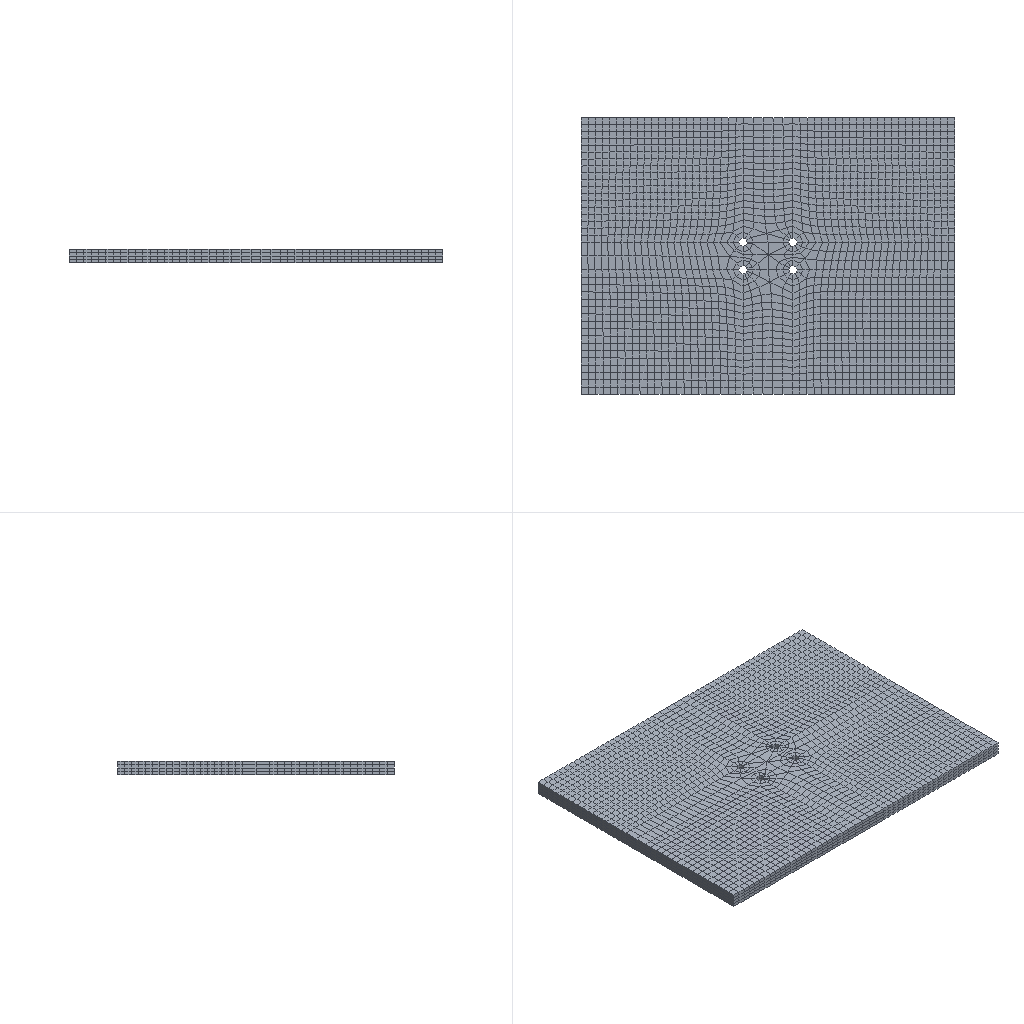Simulation study | abaqus
Set-up summary:
category,name,step,type,value,unit,region
solver,abaqus,,Abaqus/CAE 2024
units,mm-N-s-tonne (MPa),,inferred,E=200000 density=
analysis,Step-1,,static,time_period=1
analysis,Step-2,,static,time_period=1
mesh,nodes,,,10331
mesh,elements,,,7836
element_type,SC8R,,,7836
material,Material-1,,E,200000
material,Material-1,,nu,0.25
material,Material-1,,behaviors,damage initiation; elastic engineering constants
section,,,shell section,1,,CompositeLayup-1-1
load,Load-1,Step-1,pressure,1.977,,_PickedSurf10
load,Load-1-Copy,Step-1,pressure,1.995,,_PickedSurf12
load,Load-1-Copy-Copy,Step-1,pressure,1.934,,_PickedSurf13
load,Load-1-Copy-Copy-Copy,Step-1,pressure,1.945,,_PickedSurf14
load,Load-5,Step-1,pressure,1.974,,_PickedSurf15
load,Load-5-Copy,Step-1,pressure,1.945,,_PickedSurf16
load,Load-5-Copy-Copy,Step-1,pressure,1.995,,_PickedSurf17
load,Load-5-Copy-Copy-Copy,Step-1,pressure,1.934,,_PickedSurf18
bc,BC-1,Step-1,encastre,[dofs=ENCASTRE],,_PickedSet4
bc,BC-2,Step-1,fixed,"[dofs=rx,ry,rz,x,y,z n=6]",,_PickedSet9
bc,BC-2,Step-2,displacement,0.2 [dofs=x],,_PickedSet9
bc,BC-2,Step-2,fixed,"[dofs=rx,ry,rz n=3]",,_PickedSet9
constraint,coupling,,,1
Abaqus input file, long lists of numbers shortened:
*Heading
** Job name: deck Model name: Model-1-Copy-Copy
** Generated by: Abaqus/CAE 2024
*Preprint, echo=NO, model=NO, history=NO, contact=NO
**
** PARTS
**
*Part, name=Part-1
*Node
      1,         156.,         -90.,           0.
      2,         156.,         -90.,          10.
** (10328 more lines like these left out)
*Element, type=SC8R
1,   1,   4, 117, 118, 105, 110, 984, 981
2, 105, 110, 984, 981, 106, 109, 985, 982
** (7834 more lines like these left out)
*Orientation, name=Ori-1
1., 0., 0., 0., 1., 0.
3, 0.
** Region: (CompositeLayup-1-1: Generated From Layup)
*Elset, elset=CompositeLayup-1-1, generate
    1,  7836,     1
** Section: CompositeLayup-1-1
*Shell Section, elset=CompositeLayup-1-1, composite, orientation=Ori-1, stack direction=3, layup=CompositeLayup-1
1., 3, Material-1, -45., Ply-1
1., 3, Material-1, 45., Ply-2
1., 3, Material-1, -45., Ply-3
1., 3, Material-1, 45., Ply-4
*End Part
**
**
** ASSEMBLY
**
*Assembly, name=Assembly
**
*Instance, name=Part-1-1, part=Part-1
*End Instance
**
*Node
      1,         270.,        -100.,           5.
*Nset, nset=_PickedSet4, internal, instance=Part-1-1
   49,   50,   51,   52,   57,   58,   61,   63,  457,  458,  459,  460,  461,  462,  463,  464
  465,  466,  467,  468,  469,  470,  471,  472,  473,  474,  475,  476,  477,  478,  479,  480
** (10 more lines like these left out)
*Elset, elset=_PickedSet4, internal, instance=Part-1-1
 2121, 2122, 2186, 2208, 2213, 2214, 2215, 2216, 2217, 2218, 2219, 2220, 2221, 2222, 2223, 2224
 2225, 2226, 2227, 2228, 2229, 2587, 2588, 2589, 2590, 2591, 2592, 2593, 2594, 2595, 2596, 2597
** (8 more lines like these left out)
*Nset, nset=_PickedSet8, internal
 1,
*Nset, nset=_PickedSet9, internal
 1,
*Elset, elset=__PickedSurf7_S6, internal, instance=Part-1-1
   25,   26,   90,  112, 7541, 7562, 7563, 7564, 7637, 7658, 7679, 7700
*Elset, elset=__PickedSurf7_S3, internal, instance=Part-1-1
 117, 118, 119, 120, 121, 122, 123, 124, 125, 126, 127, 128, 129, 130, 131, 132
 133, 491, 492, 493, 494, 495, 496, 497, 498, 499, 500, 501, 502, 503, 504, 505
** (1 more lines like these left out)
*Elset, elset=__PickedSurf7_S5, internal, instance=Part-1-1
  899,  900,  901,  902,  903,  904,  905,  906,  907,  908,  909,  910,  911,  912,  913,  914
  915,  916,  917,  918,  919,  920,  921,  922,  923,  924,  925,  926,  927,  928,  929,  930
** (5 more lines like these left out)
*Elset, elset=__PickedSurf7_S4, internal, instance=Part-1-1, generate
 7729,  7792,    21
*Surface, type=ELEMENT, name=_PickedSurf7, internal
__PickedSurf7_S6, S6
__PickedSurf7_S3, S3
__PickedSurf7_S4, S4
__PickedSurf7_S5, S5
*Elset, elset=__PickedSurf10_S2, internal, instance=Part-1-1
 5475, 5476, 5480, 5484, 5488, 5492, 5849, 5853, 5857, 7832, 7836
*Surface, type=ELEMENT, name=_PickedSurf10, internal
__PickedSurf10_S2, S2
*Elset, elset=__PickedSurf12_S2, internal, instance=Part-1-1
 1696, 1700, 1704, 1724, 1728, 1732, 2104, 2108, 2112, 2116
*Surface, type=ELEMENT, name=_PickedSurf12, internal
__PickedSurf12_S2, S2
*Elset, elset=__PickedSurf13_S2, internal, instance=Part-1-1
    4,    8,   12,   16,   20, 1684, 1688, 1692, 1708, 1712, 1716, 1720
*Surface, type=ELEMENT, name=_PickedSurf13, internal
__PickedSurf13_S2, S2
*Elset, elset=__PickedSurf14_S2, internal, instance=Part-1-1
 5942, 5943, 5944, 7797, 7798, 7799, 7812, 7816, 7820, 7824, 7828
*Surface, type=ELEMENT, name=_PickedSurf14, internal
__PickedSurf14_S2, S2
*Elset, elset=__PickedSurf15_S1, internal, instance=Part-1-1
 5469, 5470, 5477, 5481, 5485, 5489, 5852, 5856, 5860, 7829, 7833
*Surface, type=ELEMENT, name=_PickedSurf15, internal
__PickedSurf15_S1, S1
*Elset, elset=__PickedSurf16_S1, internal, instance=Part-1-1
 5933, 5934, 5935, 7806, 7807, 7808, 7809, 7813, 7817, 7821, 7825
*Surface, type=ELEMENT, name=_PickedSurf16, internal
__PickedSurf16_S1, S1
*Elset, elset=__PickedSurf17_S1, internal, instance=Part-1-1
 1693, 1697, 1701, 1721, 1725, 1729, 2101, 2105, 2109, 2113
*Surface, type=ELEMENT, name=_PickedSurf17, internal
__PickedSurf17_S1, S1
*Elset, elset=__PickedSurf18_S1, internal, instance=Part-1-1
    1,    5,    9,   13,   17, 1681, 1685, 1689, 1705, 1709, 1713, 1717
*Surface, type=ELEMENT, name=_PickedSurf18, internal
__PickedSurf18_S1, S1
** Constraint: Constraint-1
*Coupling, constraint name=Constraint-1, ref node=_PickedSet8, surface=_PickedSurf7
*Kinematic
*End Assembly
**
** MATERIALS
**
*Material, name=Material-1
*Damage Initiation, criterion=HASHIN
2500.,  1500., 50000.,150000.,    75.,    40.
*Elastic, type=ENGINEERING CONSTANTS
200000.,10000.,10000.,  0.25,   0.4,   0.4, 6000., 6000.
 3000.,
** ----------------------------------------------------------------
**
** STEP: Step-1
**
*Step, name=Step-1, nlgeom=NO, inc=1000
*Static, stabilize=0.0002, allsdtol=0.05, continue=NO
0.1, 1., 1e-05, 0.1
**
** BOUNDARY CONDITIONS
**
** Name: BC-1 Type: Symmetry/Antisymmetry/Encastre
*Boundary
_PickedSet4, ENCASTRE
** Name: BC-2 Type: Displacement/Rotation
*Boundary
_PickedSet9, 1, 1
_PickedSet9, 2, 2
_PickedSet9, 3, 3
_PickedSet9, 4, 4
_PickedSet9, 5, 5
_PickedSet9, 6, 6
**
** LOADS
**
** Name: Load-1   Type: Pressure
*Dsload
_PickedSurf10, P, 1.977
** Name: Load-1-Copy   Type: Pressure
*Dsload
_PickedSurf12, P, 1.995
** Name: Load-1-Copy-Copy   Type: Pressure
*Dsload
_PickedSurf13, P, 1.934
** Name: Load-1-Copy-Copy-Copy   Type: Pressure
*Dsload
_PickedSurf14, P, 1.945
** Name: Load-5   Type: Pressure
*Dsload
_PickedSurf15, P, 1.974
** Name: Load-5-Copy   Type: Pressure
*Dsload
_PickedSurf16, P, 1.945
** Name: Load-5-Copy-Copy   Type: Pressure
*Dsload
_PickedSurf17, P, 1.995
** Name: Load-5-Copy-Copy-Copy   Type: Pressure
*Dsload
_PickedSurf18, P, 1.934
**
** OUTPUT REQUESTS
**
*Restart, write, frequency=0
**
** FIELD OUTPUT: F-Output-1
**
*Output, field, variable=PRESELECT
**
** HISTORY OUTPUT: H-Output-1
**
*Output, history, variable=PRESELECT
*End Step
** ----------------------------------------------------------------
**
** STEP: Step-2
**
*Step, name=Step-2, nlgeom=NO, inc=1000
*Static, stabilize=0.0002, allsdtol=0.05, continue=NO
0.1, 1., 1e-05, 0.1
**
** BOUNDARY CONDITIONS
**
** Name: BC-2 Type: Displacement/Rotation
*Boundary
_PickedSet9, 1, 1, 0.2
_PickedSet9, 4, 4
_PickedSet9, 5, 5
_PickedSet9, 6, 6
**
** OUTPUT REQUESTS
**
*Restart, write, frequency=0
**
** FIELD OUTPUT: F-Output-1
**
*Output, field, variable=PRESELECT
**
** HISTORY OUTPUT: H-Output-1
**
*Output, history, variable=PRESELECT
*End Step
Results summary:
result,odb.job_status,,,JOB_STATUS_COMPLETED_SUCCESSFULLY,"consistent, unstated (Abaqus has no unit system)"
result,steps[0].procedure,Step-1,,*STATIC,"consistent, unstated (Abaqus has no unit system)"
result,steps[0].time_period,Step-1,,1,"consistent, unstated (Abaqus has no unit system)"
result,steps[0].n_frames,Step-1,,11,"consistent, unstated (Abaqus has no unit system)"
result,steps[0].last_frame.id,Step-1,,10,"consistent, unstated (Abaqus has no unit system)"
result,steps[0].last_frame.value,Step-1,,1,"consistent, unstated (Abaqus has no unit system)"
result,steps[0].last_frame.description,Step-1,,Increment     10: Step Time =    1.000,"consistent, unstated (Abaqus has no unit system)"
result,steps[0].completed,Step-1,,True,"consistent, unstated (Abaqus has no unit system)"
result,steps[0].max_U_magnitude,Step-1,,0.0009148,"consistent, unstated (Abaqus has no unit system)"
result,steps[0].max_S_mises,Step-1,,2.861,"consistent, unstated (Abaqus has no unit system)"
result,steps[0].RF_sum[1],Step-1,,2.26498e-06,"consistent, unstated (Abaqus has no unit system)"
result,steps[0].RF_sum[2],Step-1,,-7.7486e-07,"consistent, unstated (Abaqus has no unit system)"
result,steps[0].RF_sum[3],Step-1,,-0.0002089,"consistent, unstated (Abaqus has no unit system)"
result,steps[1].procedure,Step-2,,*STATIC,"consistent, unstated (Abaqus has no unit system)"
result,steps[1].time_period,Step-2,,1,"consistent, unstated (Abaqus has no unit system)"
result,steps[1].n_frames,Step-2,,11,"consistent, unstated (Abaqus has no unit system)"
result,steps[1].last_frame.id,Step-2,,10,"consistent, unstated (Abaqus has no unit system)"
result,steps[1].last_frame.value,Step-2,,1,"consistent, unstated (Abaqus has no unit system)"
result,steps[1].last_frame.description,Step-2,,Increment     10: Step Time =    1.000,"consistent, unstated (Abaqus has no unit system)"
result,steps[1].completed,Step-2,,True,"consistent, unstated (Abaqus has no unit system)"
result,steps[1].max_U_magnitude,Step-2,,0.2,"consistent, unstated (Abaqus has no unit system)"
result,steps[1].max_S_mises,Step-2,,129.501,"consistent, unstated (Abaqus has no unit system)"
result,steps[1].RF_sum[1],Step-2,,-0.003662,"consistent, unstated (Abaqus has no unit system)"
result,steps[1].RF_sum[2],Step-2,,-0.001404,"consistent, unstated (Abaqus has no unit system)"
result,steps[1].RF_sum[3],Step-2,,-0.0002158,"consistent, unstated (Abaqus has no unit system)"